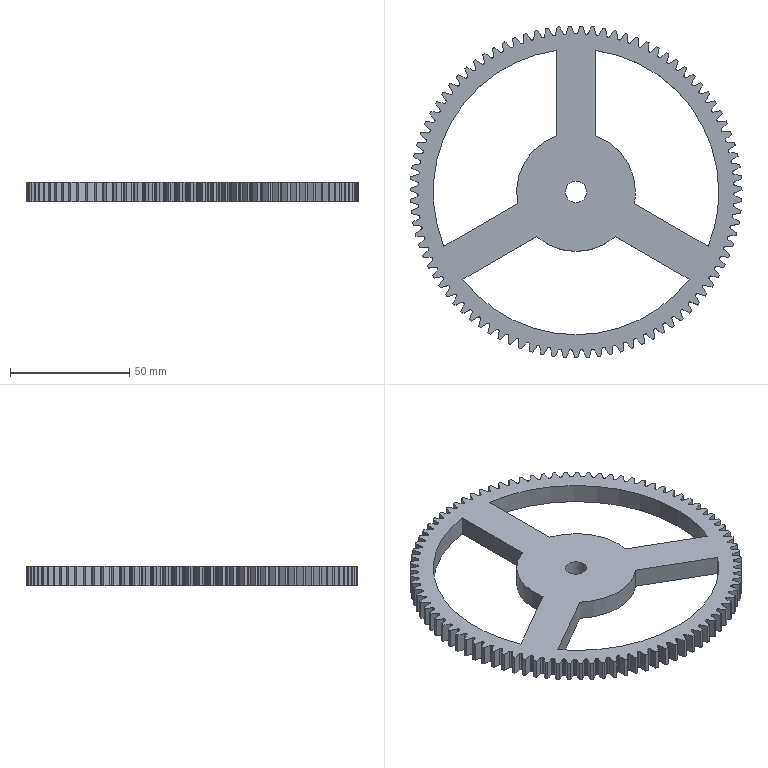Part | SolidWorks | features Extrusion 1, ICE 1 | 1 solid | 601 faces | box 139.495 x 139.48 x 8.27 mm | volume 56874 mm3 | cylinder 411 | spline 182 | plane 8 | commonest cylinder face diameters 1.14 x219 132.75 x91 139.5 x91 50 x4 120 x4 9 x2